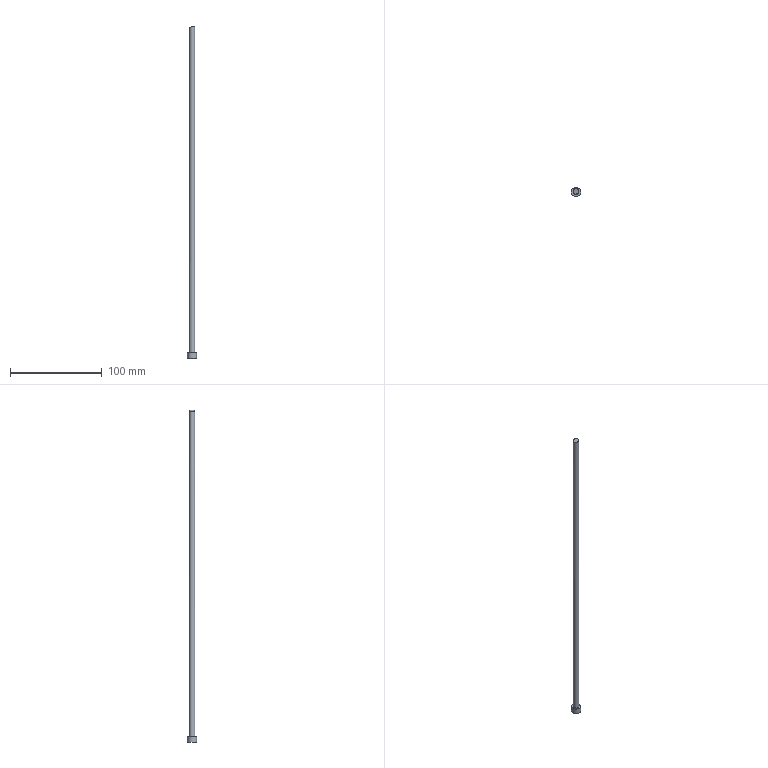Part | NX | features solid 2 | 1 solid | 5 faces | box 10 x 10 x 362.708 mm | volume 10527 mm3 | cylinder 2 | plane 2 | spline 1 | commonest cylinder face diameters 6 x1 10 x1
STEP:
#1=CARTESIAN_POINT('',(3.,31.,-339.5));
#2=VERTEX_POINT('',#1);
#3=CARTESIAN_POINT('',(0.,31.,-339.5));
#4=DIRECTION('',(0.,0.,-1.));
#5=DIRECTION('',(1.,0.,0.));
#6=AXIS2_PLACEMENT_3D('',#3,#4,#5);
#7=CIRCLE('',#6,3.);
#8=EDGE_CURVE('',#2,#2,#7,.T.);
#9=ORIENTED_EDGE('',*,*,#8,.F.);
#10=EDGE_LOOP('',(#9));
#11=FACE_BOUND('',#10,.T.);
#12=CARTESIAN_POINT('',(2.939,31.604,17.18));
#13=VERTEX_POINT('',#12);
#14=CARTESIAN_POINT('',(1.788,33.792,16.798));
#15=CARTESIAN_POINT('',(3.275,31.684,17.28));
#16=CARTESIAN_POINT('',(2.742,29.098,17.161));
#17=CARTESIAN_POINT('',(0.6075,27.75,16.525));
#18=CARTESIAN_POINT('',(-1.798,28.219,15.726));
#19=CARTESIAN_POINT('',(-3.272,30.311,15.178));
#20=CARTESIAN_POINT('',(-2.744,32.896,15.321));
#21=CARTESIAN_POINT('',(-0.6244,34.244,16.021));
#22=CARTESIAN_POINT('',(1.788,33.792,16.798));
#23=CARTESIAN_POINT('',(3.275,31.684,17.28));
#24=CARTESIAN_POINT('',(2.742,29.098,17.161));
#25=B_SPLINE_CURVE_WITH_KNOTS('',3,(#14,#15,#16,#17,#18,#19,#20,#21,#22,#23,#24),.UNSPECIFIED.,.T.,.F.,(1,1,1,1,1,1,1,1,1,1,1,1,1,1,1),(-0.007219,-0.004813,-0.002406,0.,0.002406,0.004813,0.007219,0.009625,0.01203,0.01444,0.01684,0.01925,0.02166,0.02406,0.02647),.UNSPECIFIED.);
#26=EDGE_CURVE('',#13,#13,#25,.T.);
#27=ORIENTED_EDGE('',*,*,#26,.T.);
#28=EDGE_LOOP('',(#27));
#29=FACE_BOUND('',#28,.T.);
#30=CARTESIAN_POINT('',(0.,31.,-345.5));
#31=DIRECTION('',(0.,0.,1.));
#32=DIRECTION('',(1.,0.,0.));
#33=AXIS2_PLACEMENT_3D('',#30,#31,#32);
#34=CYLINDRICAL_SURFACE('',#33,3.);
#35=ADVANCED_FACE('',(#11,#29),#34,.T.);
#36=ORIENTED_EDGE('',*,*,#8,.T.);
#37=EDGE_LOOP('',(#36));
#38=FACE_BOUND('',#37,.T.);
#39=CARTESIAN_POINT('',(5.,31.,-339.5));
#40=VERTEX_POINT('',#39);
#41=CARTESIAN_POINT('',(0.,31.,-339.5));
#42=DIRECTION('',(0.,0.,1.));
#43=DIRECTION('',(1.,0.,0.));
#44=AXIS2_PLACEMENT_3D('',#41,#42,#43);
#45=CIRCLE('',#44,5.);
#46=EDGE_CURVE('',#40,#40,#45,.T.);
#47=ORIENTED_EDGE('',*,*,#46,.T.);
#48=EDGE_LOOP('',(#47));
#49=FACE_BOUND('',#48,.T.);
#50=CARTESIAN_POINT('',(0.,31.,-339.5));
#51=DIRECTION('',(0.,0.,1.));
#52=DIRECTION('',(1.,0.,0.));
#53=AXIS2_PLACEMENT_3D('',#50,#51,#52);
#54=PLANE('',#53);
#55=ADVANCED_FACE('',(#38,#49),#54,.T.);
#56=CARTESIAN_POINT('',(5.,31.,-345.5));
#57=VERTEX_POINT('',#56);
#58=CARTESIAN_POINT('',(0.,31.,-345.5));
#59=DIRECTION('',(0.,0.,-1.));
#60=DIRECTION('',(1.,0.,0.));
#61=AXIS2_PLACEMENT_3D('',#58,#59,#60);
#62=CIRCLE('',#61,5.);
#63=EDGE_CURVE('',#57,#57,#62,.T.);
#64=ORIENTED_EDGE('',*,*,#63,.T.);
#65=EDGE_LOOP('',(#64));
#66=FACE_BOUND('',#65,.T.);
#67=CARTESIAN_POINT('',(0.,31.,-345.5));
#68=DIRECTION('',(0.,0.,-1.));
#69=DIRECTION('',(-1.,0.,0.));
#70=AXIS2_PLACEMENT_3D('',#67,#68,#69);
#71=PLANE('',#70);
#72=ADVANCED_FACE('',(#66),#71,.T.);
#73=ORIENTED_EDGE('',*,*,#46,.F.);
#74=EDGE_LOOP('',(#73));
#75=FACE_BOUND('',#74,.T.);
#76=ORIENTED_EDGE('',*,*,#63,.F.);
#77=EDGE_LOOP('',(#76));
#78=FACE_BOUND('',#77,.T.);
#79=CARTESIAN_POINT('',(0.,31.,-345.5));
#80=DIRECTION('',(0.,0.,1.));
#81=DIRECTION('',(1.,0.,0.));
#82=AXIS2_PLACEMENT_3D('',#79,#80,#81);
#83=CYLINDRICAL_SURFACE('',#82,5.);
#84=ADVANCED_FACE('',(#75,#78),#83,.T.);
#85=ORIENTED_EDGE('',*,*,#26,.F.);
#86=EDGE_LOOP('',(#85));
#87=FACE_BOUND('',#86,.T.);
#88=CARTESIAN_POINT('',(-3.05,27.945,15.294));
#89=CARTESIAN_POINT('',(-3.045,29.981,15.263));
#90=CARTESIAN_POINT('',(-3.04,32.018,15.231));
#91=CARTESIAN_POINT('',(-3.034,34.054,15.198));
#92=CARTESIAN_POINT('',(-1.034,27.945,15.997));
#93=CARTESIAN_POINT('',(-1.029,29.982,15.967));
#94=CARTESIAN_POINT('',(-1.024,32.018,15.935));
#95=CARTESIAN_POINT('',(-1.019,34.055,15.902));
#96=CARTESIAN_POINT('',(0.9998,27.946,16.654));
#97=CARTESIAN_POINT('',(1.004,29.982,16.624));
#98=CARTESIAN_POINT('',(1.009,32.019,16.593));
#99=CARTESIAN_POINT('',(1.014,34.055,16.56));
#100=CARTESIAN_POINT('',(3.047,27.946,17.269));
#101=CARTESIAN_POINT('',(3.051,29.983,17.239));
#102=CARTESIAN_POINT('',(3.056,32.019,17.209));
#103=CARTESIAN_POINT('',(3.06,34.056,17.177));
#104=B_SPLINE_SURFACE_WITH_KNOTS('',3,3,((#88,#89,#90,#91),(#92,#93,#94,#95),(#96,#97,#98,#99),(#100,#101,#102,#103)),.UNSPECIFIED.,.F.,.F.,.F.,(4,4),(4,4),(0.6301,0.6624),(0.08232,0.1983),.PIECEWISE_BEZIER_KNOTS.);
#105=ADVANCED_FACE('',(#87),#104,.T.);
#106=CLOSED_SHELL('',(#35,#55,#72,#84,#105));
#107=MANIFOLD_SOLID_BREP('',#106);
#108=(LENGTH_UNIT()NAMED_UNIT(*)SI_UNIT(.MILLI.,.METRE.));
#109=UNCERTAINTY_MEASURE_WITH_UNIT(LENGTH_MEASURE(0.0508),#108,'','');
#110=(NAMED_UNIT(*)PLANE_ANGLE_UNIT()SI_UNIT($,.RADIAN.));
#111=(NAMED_UNIT(*)SI_UNIT($,.STERADIAN.)SOLID_ANGLE_UNIT());
#112=(GEOMETRIC_REPRESENTATION_CONTEXT(3)GLOBAL_UNCERTAINTY_ASSIGNED_CONTEXT((#109))GLOBAL_UNIT_ASSIGNED_CONTEXT((#108,#110,#111))REPRESENTATION_CONTEXT('',''));
#113=ADVANCED_BREP_SHAPE_REPRESENTATION('',(#107),#112);